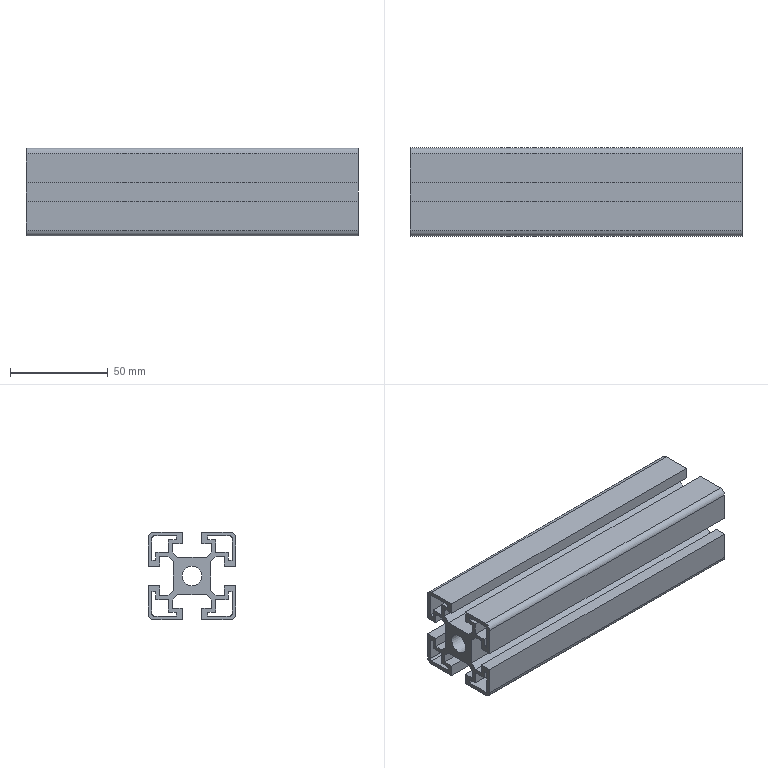Part | STEP file | 1_15 | 1 solid | 87 faces | box 170 x 45 x 45 mm | volume 139016 mm3 | plane 78 | cylinder 9 | commonest cylinder face diameters 2 x4 6 x4 10 x1